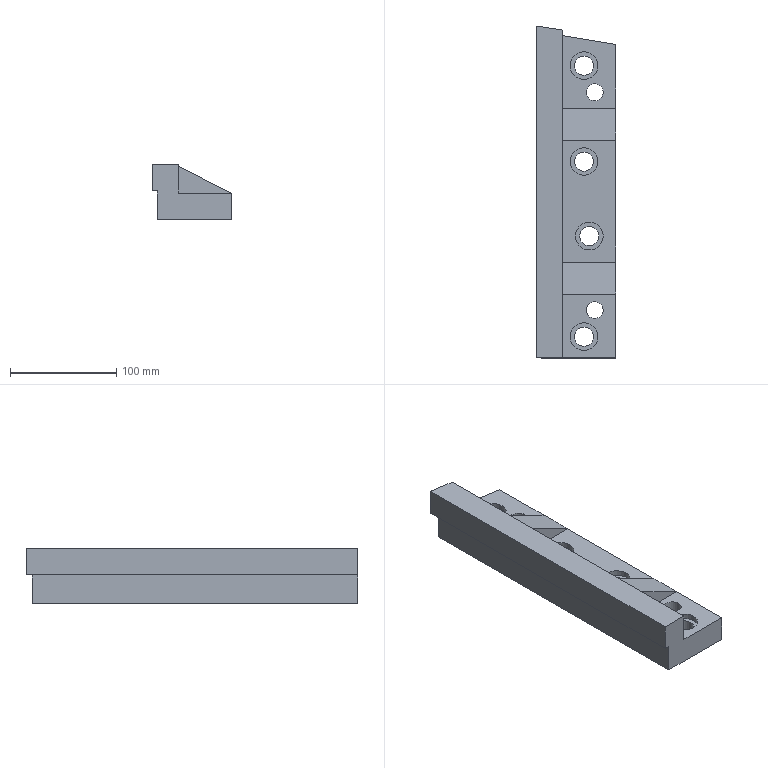Part | NX | features solid 2 | 1 solid | 33 faces | box 75 x 311.68 x 52 mm | volume 727777 mm3 | plane 21 | cylinder 10 | spline 2 | commonest cylinder face diameters 18 x4 26 x4 16 x2
STEP:
#1=CARTESIAN_POINT('',(-267.,-375.538,-30.));
#2=VERTEX_POINT('',#1);
#3=CARTESIAN_POINT('',(-280.,-375.538,-30.));
#4=DIRECTION('',(0.,0.,-1.));
#5=DIRECTION('',(1.,0.,0.));
#6=AXIS2_PLACEMENT_3D('',#3,#4,#5);
#7=CIRCLE('',#6,13.);
#8=EDGE_CURVE('',#2,#2,#7,.T.);
#9=ORIENTED_EDGE('',*,*,#8,.T.);
#10=EDGE_LOOP('',(#9));
#11=FACE_BOUND('',#10,.T.);
#12=CARTESIAN_POINT('',(-262.,-445.538,-30.));
#13=VERTEX_POINT('',#12);
#14=CARTESIAN_POINT('',(-275.,-445.538,-30.));
#15=DIRECTION('',(0.,0.,-1.));
#16=DIRECTION('',(1.,0.,0.));
#17=AXIS2_PLACEMENT_3D('',#14,#15,#16);
#18=CIRCLE('',#17,13.);
#19=EDGE_CURVE('',#13,#13,#18,.T.);
#20=ORIENTED_EDGE('',*,*,#19,.T.);
#21=EDGE_LOOP('',(#20));
#22=FACE_BOUND('',#21,.T.);
#23=CARTESIAN_POINT('',(-250.,-470.,-30.));
#24=VERTEX_POINT('',#23);
#25=CARTESIAN_POINT('',(-250.,-355.538,-30.));
#26=VERTEX_POINT('',#25);
#27=CARTESIAN_POINT('',(-250.,-560.,-30.));
#28=DIRECTION('',(0.,1.,0.));
#29=VECTOR('',#28,1000.);
#30=LINE('',#27,#29);
#31=EDGE_CURVE('',#24,#26,#30,.T.);
#32=ORIENTED_EDGE('',*,*,#31,.T.);
#33=CARTESIAN_POINT('',(-300.,-355.538,-30.));
#34=VERTEX_POINT('',#33);
#35=CARTESIAN_POINT('',(-300.,-355.538,-30.));
#36=DIRECTION('',(1.,0.,0.));
#37=VECTOR('',#36,1000.);
#38=LINE('',#35,#37);
#39=EDGE_CURVE('',#34,#26,#38,.T.);
#40=ORIENTED_EDGE('',*,*,#39,.F.);
#41=CARTESIAN_POINT('',(-300.,-470.,-30.));
#42=VERTEX_POINT('',#41);
#43=CARTESIAN_POINT('',(-300.,-560.,-30.));
#44=DIRECTION('',(0.,1.,0.));
#45=VECTOR('',#44,1000.);
#46=LINE('',#43,#45);
#47=EDGE_CURVE('',#42,#34,#46,.T.);
#48=ORIENTED_EDGE('',*,*,#47,.F.);
#49=CARTESIAN_POINT('',(-300.,-470.,-30.));
#50=DIRECTION('',(1.,0.,0.));
#51=VECTOR('',#50,1000.);
#52=LINE('',#49,#51);
#53=EDGE_CURVE('',#42,#24,#52,.T.);
#54=ORIENTED_EDGE('',*,*,#53,.T.);
#55=EDGE_LOOP('',(#32,#40,#48,#54));
#56=FACE_BOUND('',#55,.T.);
#57=CARTESIAN_POINT('',(-272.356,-257.29,-30.));
#58=DIRECTION('',(0.,0.,-1.));
#59=DIRECTION('',(-1.,0.,0.));
#60=AXIS2_PLACEMENT_3D('',#57,#58,#59);
#61=PLANE('',#60);
#62=ADVANCED_FACE('',(#11,#22,#56),#61,.F.);
#63=CARTESIAN_POINT('',(-267.,-285.538,-30.));
#64=VERTEX_POINT('',#63);
#65=CARTESIAN_POINT('',(-280.,-285.538,-30.));
#66=DIRECTION('',(0.,0.,-1.));
#67=DIRECTION('',(1.,0.,0.));
#68=AXIS2_PLACEMENT_3D('',#65,#66,#67);
#69=CIRCLE('',#68,13.);
#70=EDGE_CURVE('',#64,#64,#69,.T.);
#71=ORIENTED_EDGE('',*,*,#70,.T.);
#72=EDGE_LOOP('',(#71));
#73=FACE_BOUND('',#72,.T.);
#74=CARTESIAN_POINT('',(-262.,-310.538,-30.));
#75=VERTEX_POINT('',#74);
#76=CARTESIAN_POINT('',(-270.,-310.538,-30.));
#77=DIRECTION('',(0.,0.,-1.));
#78=DIRECTION('',(1.,0.,0.));
#79=AXIS2_PLACEMENT_3D('',#76,#77,#78);
#80=CIRCLE('',#79,8.);
#81=EDGE_CURVE('',#75,#75,#80,.T.);
#82=ORIENTED_EDGE('',*,*,#81,.T.);
#83=EDGE_LOOP('',(#82));
#84=FACE_BOUND('',#83,.T.);
#85=CARTESIAN_POINT('',(-300.,-325.538,-30.));
#86=VERTEX_POINT('',#85);
#87=CARTESIAN_POINT('',(-300.,-257.2,-30.));
#88=VERTEX_POINT('',#87);
#89=CARTESIAN_POINT('',(-300.,-560.,-30.));
#90=DIRECTION('',(0.,1.,0.));
#91=VECTOR('',#90,1000.);
#92=LINE('',#89,#91);
#93=EDGE_CURVE('',#86,#88,#92,.T.);
#94=ORIENTED_EDGE('',*,*,#93,.F.);
#95=CARTESIAN_POINT('',(-250.,-325.538,-30.));
#96=VERTEX_POINT('',#95);
#97=CARTESIAN_POINT('',(-300.,-325.538,-30.));
#98=DIRECTION('',(1.,0.,0.));
#99=VECTOR('',#98,1000.);
#100=LINE('',#97,#99);
#101=EDGE_CURVE('',#86,#96,#100,.T.);
#102=ORIENTED_EDGE('',*,*,#101,.T.);
#103=CARTESIAN_POINT('',(-250.,-265.538,-30.));
#104=VERTEX_POINT('',#103);
#105=CARTESIAN_POINT('',(-250.,-560.,-30.));
#106=DIRECTION('',(0.,1.,0.));
#107=VECTOR('',#106,1000.);
#108=LINE('',#105,#107);
#109=EDGE_CURVE('',#96,#104,#108,.T.);
#110=ORIENTED_EDGE('',*,*,#109,.T.);
#111=CARTESIAN_POINT('',(-250.,-265.538,-30.));
#112=CARTESIAN_POINT('',(-266.667,-262.759,-30.));
#113=CARTESIAN_POINT('',(-283.333,-259.979,-30.));
#114=CARTESIAN_POINT('',(-300.,-257.2,-30.));
#115=B_SPLINE_CURVE_WITH_KNOTS('',3,(#111,#112,#113,#114),.UNSPECIFIED.,.F.,.F.,(4,4),(0.3169,0.3676),.UNSPECIFIED.);
#116=EDGE_CURVE('',#104,#88,#115,.T.);
#117=ORIENTED_EDGE('',*,*,#116,.T.);
#118=EDGE_LOOP('',(#94,#102,#110,#117));
#119=FACE_BOUND('',#118,.T.);
#120=CARTESIAN_POINT('',(-272.356,-257.29,-30.));
#121=DIRECTION('',(0.,0.,-1.));
#122=DIRECTION('',(-1.,0.,0.));
#123=AXIS2_PLACEMENT_3D('',#120,#121,#122);
#124=PLANE('',#123);
#125=ADVANCED_FACE('',(#73,#84,#119),#124,.F.);
#126=CARTESIAN_POINT('',(-250.,-560.,-30.));
#127=VERTEX_POINT('',#126);
#128=CARTESIAN_POINT('',(-250.,-500.,-30.));
#129=VERTEX_POINT('',#128);
#130=CARTESIAN_POINT('',(-250.,-560.,-30.));
#131=DIRECTION('',(0.,1.,0.));
#132=VECTOR('',#131,1000.);
#133=LINE('',#130,#132);
#134=EDGE_CURVE('',#127,#129,#133,.T.);
#135=ORIENTED_EDGE('',*,*,#134,.T.);
#136=CARTESIAN_POINT('',(-300.,-500.,-30.));
#137=VERTEX_POINT('',#136);
#138=CARTESIAN_POINT('',(-300.,-500.,-30.));
#139=DIRECTION('',(1.,0.,0.));
#140=VECTOR('',#139,1000.);
#141=LINE('',#138,#140);
#142=EDGE_CURVE('',#137,#129,#141,.T.);
#143=ORIENTED_EDGE('',*,*,#142,.F.);
#144=CARTESIAN_POINT('',(-300.,-560.,-30.));
#145=VERTEX_POINT('',#144);
#146=CARTESIAN_POINT('',(-300.,-560.,-30.));
#147=DIRECTION('',(0.,1.,0.));
#148=VECTOR('',#147,1000.);
#149=LINE('',#146,#148);
#150=EDGE_CURVE('',#145,#137,#149,.T.);
#151=ORIENTED_EDGE('',*,*,#150,.F.);
#152=CARTESIAN_POINT('',(-245.,-560.,-30.));
#153=DIRECTION('',(-1.,0.,0.));
#154=VECTOR('',#153,1000.);
#155=LINE('',#152,#154);
#156=EDGE_CURVE('',#127,#145,#155,.T.);
#157=ORIENTED_EDGE('',*,*,#156,.F.);
#158=EDGE_LOOP('',(#135,#143,#151,#157));
#159=FACE_BOUND('',#158,.T.);
#160=CARTESIAN_POINT('',(-262.,-515.,-30.));
#161=VERTEX_POINT('',#160);
#162=CARTESIAN_POINT('',(-270.,-515.,-30.));
#163=DIRECTION('',(0.,0.,1.));
#164=DIRECTION('',(1.,0.,0.));
#165=AXIS2_PLACEMENT_3D('',#162,#163,#164);
#166=CIRCLE('',#165,8.);
#167=EDGE_CURVE('',#161,#161,#166,.T.);
#168=ORIENTED_EDGE('',*,*,#167,.F.);
#169=EDGE_LOOP('',(#168));
#170=FACE_BOUND('',#169,.T.);
#171=CARTESIAN_POINT('',(-267.,-540.,-30.));
#172=VERTEX_POINT('',#171);
#173=CARTESIAN_POINT('',(-280.,-540.,-30.));
#174=DIRECTION('',(0.,0.,1.));
#175=DIRECTION('',(1.,0.,0.));
#176=AXIS2_PLACEMENT_3D('',#173,#174,#175);
#177=CIRCLE('',#176,13.);
#178=EDGE_CURVE('',#172,#172,#177,.T.);
#179=ORIENTED_EDGE('',*,*,#178,.F.);
#180=EDGE_LOOP('',(#179));
#181=FACE_BOUND('',#180,.T.);
#182=CARTESIAN_POINT('',(-272.356,-257.29,-30.));
#183=DIRECTION('',(0.,0.,-1.));
#184=DIRECTION('',(-1.,0.,0.));
#185=AXIS2_PLACEMENT_3D('',#182,#183,#184);
#186=PLANE('',#185);
#187=ADVANCED_FACE('',(#159,#170,#181),#186,.F.);
#188=CARTESIAN_POINT('',(-289.,-540.,-55.));
#189=VERTEX_POINT('',#188);
#190=CARTESIAN_POINT('',(-280.,-540.,-55.));
#191=DIRECTION('',(0.,0.,-1.));
#192=DIRECTION('',(-1.,0.,0.));
#193=AXIS2_PLACEMENT_3D('',#190,#191,#192);
#194=CIRCLE('',#193,9.);
#195=EDGE_CURVE('',#189,#189,#194,.T.);
#196=ORIENTED_EDGE('',*,*,#195,.T.);
#197=EDGE_LOOP('',(#196));
#198=FACE_BOUND('',#197,.T.);
#199=CARTESIAN_POINT('',(-271.,-540.,-35.));
#200=VERTEX_POINT('',#199);
#201=CARTESIAN_POINT('',(-280.,-540.,-35.));
#202=DIRECTION('',(0.,0.,1.));
#203=DIRECTION('',(1.,0.,0.));
#204=AXIS2_PLACEMENT_3D('',#201,#202,#203);
#205=CIRCLE('',#204,9.);
#206=EDGE_CURVE('',#200,#200,#205,.F.);
#207=ORIENTED_EDGE('',*,*,#206,.F.);
#208=EDGE_LOOP('',(#207));
#209=FACE_BOUND('',#208,.T.);
#210=CARTESIAN_POINT('',(-280.,-540.,-60.));
#211=DIRECTION('',(0.,0.,1.));
#212=DIRECTION('',(1.,0.,0.));
#213=AXIS2_PLACEMENT_3D('',#210,#211,#212);
#214=CYLINDRICAL_SURFACE('',#213,9.);
#215=ADVANCED_FACE('',(#198,#209),#214,.F.);
#216=ORIENTED_EDGE('',*,*,#195,.F.);
#217=EDGE_LOOP('',(#216));
#218=FACE_BOUND('',#217,.T.);
#219=CARTESIAN_POINT('',(-278.,-515.,-55.));
#220=VERTEX_POINT('',#219);
#221=CARTESIAN_POINT('',(-270.,-515.,-55.));
#222=DIRECTION('',(0.,0.,-1.));
#223=DIRECTION('',(-1.,0.,0.));
#224=AXIS2_PLACEMENT_3D('',#221,#222,#223);
#225=CIRCLE('',#224,8.);
#226=EDGE_CURVE('',#220,#220,#225,.T.);
#227=ORIENTED_EDGE('',*,*,#226,.F.);
#228=EDGE_LOOP('',(#227));
#229=FACE_BOUND('',#228,.T.);
#230=CARTESIAN_POINT('',(-289.,-375.538,-55.));
#231=VERTEX_POINT('',#230);
#232=CARTESIAN_POINT('',(-280.,-375.538,-55.));
#233=DIRECTION('',(0.,0.,-1.));
#234=DIRECTION('',(-1.,0.,0.));
#235=AXIS2_PLACEMENT_3D('',#232,#233,#234);
#236=CIRCLE('',#235,9.);
#237=EDGE_CURVE('',#231,#231,#236,.F.);
#238=ORIENTED_EDGE('',*,*,#237,.T.);
#239=EDGE_LOOP('',(#238));
#240=FACE_BOUND('',#239,.T.);
#241=CARTESIAN_POINT('',(-289.,-285.538,-55.));
#242=VERTEX_POINT('',#241);
#243=CARTESIAN_POINT('',(-280.,-285.538,-55.));
#244=DIRECTION('',(0.,0.,-1.));
#245=DIRECTION('',(-1.,0.,0.));
#246=AXIS2_PLACEMENT_3D('',#243,#244,#245);
#247=CIRCLE('',#246,9.);
#248=EDGE_CURVE('',#242,#242,#247,.F.);
#249=ORIENTED_EDGE('',*,*,#248,.T.);
#250=EDGE_LOOP('',(#249));
#251=FACE_BOUND('',#250,.T.);
#252=CARTESIAN_POINT('',(-250.,-265.538,-55.));
#253=VERTEX_POINT('',#252);
#254=CARTESIAN_POINT('',(-320.,-254.082,-55.));
#255=VERTEX_POINT('',#254);
#256=CARTESIAN_POINT('',(-320.,-254.082,-55.));
#257=CARTESIAN_POINT('',(-318.477,-254.303,-55.));
#258=CARTESIAN_POINT('',(-315.46,-254.747,-55.));
#259=CARTESIAN_POINT('',(-311.763,-255.309,-55.));
#260=CARTESIAN_POINT('',(-308.848,-255.763,-55.));
#261=CARTESIAN_POINT('',(-306.685,-256.105,-55.));
#262=CARTESIAN_POINT('',(-304.9,-256.392,-55.));
#263=CARTESIAN_POINT('',(-303.484,-256.623,-55.));
#264=CARTESIAN_POINT('',(-302.6,-256.768,-55.));
#265=CARTESIAN_POINT('',(-301.992,-256.868,-55.));
#266=CARTESIAN_POINT('',(-301.633,-256.928,-55.));
#267=CARTESIAN_POINT('',(-301.436,-256.96,-55.));
#268=CARTESIAN_POINT('',(-301.216,-256.997,-55.));
#269=CARTESIAN_POINT('',(-301.227,-256.995,-55.));
#270=CARTESIAN_POINT('',(-301.202,-256.999,-55.));
#271=CARTESIAN_POINT('',(-301.151,-257.008,-55.));
#272=CARTESIAN_POINT('',(-300.987,-257.035,-55.));
#273=CARTESIAN_POINT('',(-300.565,-257.106,-55.));
#274=CARTESIAN_POINT('',(-299.722,-257.246,-55.));
#275=CARTESIAN_POINT('',(-298.214,-257.498,-55.));
#276=CARTESIAN_POINT('',(-296.206,-257.832,-55.));
#277=CARTESIAN_POINT('',(-293.699,-258.251,-55.));
#278=CARTESIAN_POINT('',(-291.193,-258.668,-55.));
#279=CARTESIAN_POINT('',(-288.94,-259.044,-55.));
#280=CARTESIAN_POINT('',(-287.122,-259.347,-55.));
#281=CARTESIAN_POINT('',(-285.514,-259.615,-55.));
#282=CARTESIAN_POINT('',(-284.14,-259.845,-55.));
#283=CARTESIAN_POINT('',(-283.314,-259.982,-55.));
#284=CARTESIAN_POINT('',(-282.503,-260.118,-55.));
#285=CARTESIAN_POINT('',(-282.171,-260.173,-55.));
#286=CARTESIAN_POINT('',(-281.513,-260.283,-55.));
#287=CARTESIAN_POINT('',(-280.252,-260.493,-55.));
#288=CARTESIAN_POINT('',(-278.422,-260.798,-55.));
#289=CARTESIAN_POINT('',(-276.238,-261.162,-55.));
#290=CARTESIAN_POINT('',(-274.051,-261.527,-55.));
#291=CARTESIAN_POINT('',(-271.136,-262.013,-55.));
#292=CARTESIAN_POINT('',(-267.492,-262.621,-55.));
#293=CARTESIAN_POINT('',(-263.119,-263.35,-55.));
#294=CARTESIAN_POINT('',(-257.288,-264.323,-55.));
#295=CARTESIAN_POINT('',(-252.915,-265.052,-55.));
#296=CARTESIAN_POINT('',(-250.,-265.538,-55.));
#297=B_SPLINE_CURVE_WITH_KNOTS('',3,(#256,#257,#258,#259,#260,#261,#262,#263,#264,#265,#266,#267,#268,#269,#270,#271,#272,#273,#274,#275,#276,#277,#278,#279,#280,#281,#282,#283,#284,#285,#286,#287,#288,#289,#290,#291,#292,#293,#294,#295,#296),.UNSPECIFIED.,.F.,.F.,(4,1,1,1,1,1,1,1,1,1,1,1,1,1,1,1,1,1,1,1,1,1,1,1,1,1,1,1,1,1,1,1,1,1,1,1,1,1,4),(0.,0.05833,0.1167,0.1458,0.175,0.2042,0.2187,0.2333,0.2406,0.2443,0.2479,0.2497,0.2516,0.2552,0.2625,0.2771,0.2917,0.3208,0.35,0.3792,0.4083,0.4375,0.4521,0.4667,0.4812,0.4885,0.4958,0.4995,0.5031,0.5104,0.525,0.5541,0.5833,0.6125,0.6416,0.7,0.7583,0.8166,0.9333),.UNSPECIFIED.);
#298=EDGE_CURVE('',#253,#255,#297,.F.);
#299=ORIENTED_EDGE('',*,*,#298,.F.);
#300=CARTESIAN_POINT('',(-250.,-560.,-55.));
#301=VERTEX_POINT('',#300);
#302=CARTESIAN_POINT('',(-250.,-560.,-55.));
#303=DIRECTION('',(0.,1.,0.));
#304=VECTOR('',#303,1000.);
#305=LINE('',#302,#304);
#306=EDGE_CURVE('',#301,#253,#305,.T.);
#307=ORIENTED_EDGE('',*,*,#306,.F.);
#308=CARTESIAN_POINT('',(-320.,-560.,-55.));
#309=VERTEX_POINT('',#308);
#310=CARTESIAN_POINT('',(-245.,-560.,-55.));
#311=DIRECTION('',(-1.,0.,0.));
#312=VECTOR('',#311,1000.);
#313=LINE('',#310,#312);
#314=EDGE_CURVE('',#301,#309,#313,.T.);
#315=ORIENTED_EDGE('',*,*,#314,.T.);
#316=CARTESIAN_POINT('',(-320.,-257.29,-55.));
#317=DIRECTION('',(0.,1.,0.));
#318=VECTOR('',#317,1000.);
#319=LINE('',#316,#318);
#320=EDGE_CURVE('',#309,#255,#319,.T.);
#321=ORIENTED_EDGE('',*,*,#320,.T.);
#322=EDGE_LOOP('',(#299,#307,#315,#321));
#323=FACE_BOUND('',#322,.T.);
#324=CARTESIAN_POINT('',(-278.,-310.538,-55.));
#325=VERTEX_POINT('',#324);
#326=CARTESIAN_POINT('',(-270.,-310.538,-55.));
#327=DIRECTION('',(0.,0.,-1.));
#328=DIRECTION('',(-1.,0.,0.));
#329=AXIS2_PLACEMENT_3D('',#326,#327,#328);
#330=CIRCLE('',#329,8.);
#331=EDGE_CURVE('',#325,#325,#330,.F.);
#332=ORIENTED_EDGE('',*,*,#331,.T.);
#333=EDGE_LOOP('',(#332));
#334=FACE_BOUND('',#333,.T.);
#335=CARTESIAN_POINT('',(-284.,-445.538,-55.));
#336=VERTEX_POINT('',#335);
#337=CARTESIAN_POINT('',(-275.,-445.538,-55.));
#338=DIRECTION('',(0.,0.,-1.));
#339=DIRECTION('',(-1.,0.,0.));
#340=AXIS2_PLACEMENT_3D('',#337,#338,#339);
#341=CIRCLE('',#340,9.);
#342=EDGE_CURVE('',#336,#336,#341,.F.);
#343=ORIENTED_EDGE('',*,*,#342,.T.);
#344=EDGE_LOOP('',(#343));
#345=FACE_BOUND('',#344,.T.);
#346=CARTESIAN_POINT('',(-272.356,-257.29,-55.));
#347=DIRECTION('',(0.,0.,-1.));
#348=DIRECTION('',(-1.,0.,0.));
#349=AXIS2_PLACEMENT_3D('',#346,#347,#348);
#350=PLANE('',#349);
#351=ADVANCED_FACE('',(#218,#229,#240,#251,#323,#334,#345),#350,.T.);
#352=CARTESIAN_POINT('',(-320.,-560.,-28.));
#353=VERTEX_POINT('',#352);
#354=CARTESIAN_POINT('',(-320.,-560.,-53.));
#355=DIRECTION('',(0.,0.,1.));
#356=VECTOR('',#355,1000.);
#357=LINE('',#354,#356);
#358=EDGE_CURVE('',#309,#353,#357,.T.);
#359=ORIENTED_EDGE('',*,*,#358,.F.);
#360=ORIENTED_EDGE('',*,*,#314,.F.);
#361=CARTESIAN_POINT('',(-250.,-560.,-53.));
#362=DIRECTION('',(0.,0.,1.));
#363=VECTOR('',#362,1000.);
#364=LINE('',#361,#363);
#365=EDGE_CURVE('',#301,#127,#364,.T.);
#366=ORIENTED_EDGE('',*,*,#365,.T.);
#367=ORIENTED_EDGE('',*,*,#156,.T.);
#368=CARTESIAN_POINT('',(-300.,-560.,-3.));
#369=VERTEX_POINT('',#368);
#370=CARTESIAN_POINT('',(-300.,-560.,-53.));
#371=DIRECTION('',(0.,0.,1.));
#372=VECTOR('',#371,1000.);
#373=LINE('',#370,#372);
#374=EDGE_CURVE('',#145,#369,#373,.T.);
#375=ORIENTED_EDGE('',*,*,#374,.T.);
#376=CARTESIAN_POINT('',(-325.,-560.,-3.));
#377=VERTEX_POINT('',#376);
#378=CARTESIAN_POINT('',(-300.,-560.,-3.));
#379=DIRECTION('',(-1.,0.,0.));
#380=VECTOR('',#379,1000.);
#381=LINE('',#378,#380);
#382=EDGE_CURVE('',#369,#377,#381,.T.);
#383=ORIENTED_EDGE('',*,*,#382,.T.);
#384=CARTESIAN_POINT('',(-325.,-560.,-28.));
#385=VERTEX_POINT('',#384);
#386=CARTESIAN_POINT('',(-325.,-560.,-53.));
#387=DIRECTION('',(0.,0.,1.));
#388=VECTOR('',#387,1000.);
#389=LINE('',#386,#388);
#390=EDGE_CURVE('',#385,#377,#389,.T.);
#391=ORIENTED_EDGE('',*,*,#390,.F.);
#392=CARTESIAN_POINT('',(-300.,-560.,-28.));
#393=DIRECTION('',(-1.,0.,0.));
#394=VECTOR('',#393,1000.);
#395=LINE('',#392,#394);
#396=EDGE_CURVE('',#353,#385,#395,.T.);
#397=ORIENTED_EDGE('',*,*,#396,.F.);
#398=EDGE_LOOP('',(#359,#360,#366,#367,#375,#383,#391,#397));
#399=FACE_BOUND('',#398,.T.);
#400=CARTESIAN_POINT('',(-245.,-560.,-53.));
#401=DIRECTION('',(0.,1.,0.));
#402=DIRECTION('',(0.,0.,1.));
#403=AXIS2_PLACEMENT_3D('',#400,#401,#402);
#404=PLANE('',#403);
#405=ADVANCED_FACE('',(#399),#404,.F.);
#406=CARTESIAN_POINT('',(-325.,-248.32,-28.));
#407=VERTEX_POINT('',#406);
#408=CARTESIAN_POINT('',(-325.,-248.32,-3.));
#409=VERTEX_POINT('',#408);
#410=CARTESIAN_POINT('',(-325.,-248.32,-53.));
#411=DIRECTION('',(0.,0.,1.));
#412=VECTOR('',#411,1000.);
#413=LINE('',#410,#412);
#414=EDGE_CURVE('',#407,#409,#413,.T.);
#415=ORIENTED_EDGE('',*,*,#414,.F.);
#416=CARTESIAN_POINT('',(-325.,-560.,-28.));
#417=DIRECTION('',(0.,1.,0.));
#418=VECTOR('',#417,1000.);
#419=LINE('',#416,#418);
#420=EDGE_CURVE('',#385,#407,#419,.T.);
#421=ORIENTED_EDGE('',*,*,#420,.F.);
#422=ORIENTED_EDGE('',*,*,#390,.T.);
#423=CARTESIAN_POINT('',(-325.,-560.,-3.));
#424=DIRECTION('',(0.,1.,0.));
#425=VECTOR('',#424,1000.);
#426=LINE('',#423,#425);
#427=EDGE_CURVE('',#377,#409,#426,.T.);
#428=ORIENTED_EDGE('',*,*,#427,.T.);
#429=EDGE_LOOP('',(#415,#421,#422,#428));
#430=FACE_BOUND('',#429,.T.);
#431=CARTESIAN_POINT('',(-325.,-560.,-53.));
#432=DIRECTION('',(1.,0.,0.));
#433=DIRECTION('',(0.,0.,-1.));
#434=AXIS2_PLACEMENT_3D('',#431,#432,#433);
#435=PLANE('',#434);
#436=ADVANCED_FACE('',(#430),#435,.F.);
#437=CARTESIAN_POINT('',(-250.,-265.538,-42.5));
#438=DIRECTION('',(0.,0.,-1.));
#439=VECTOR('',#438,1000.);
#440=LINE('',#437,#439);
#441=EDGE_CURVE('',#104,#253,#440,.T.);
#442=ORIENTED_EDGE('',*,*,#441,.F.);
#443=ORIENTED_EDGE('',*,*,#109,.F.);
#444=CARTESIAN_POINT('',(-250.,-355.538,-30.));
#445=DIRECTION('',(0.,1.,0.));
#446=VECTOR('',#445,1000.);
#447=LINE('',#444,#446);
#448=EDGE_CURVE('',#26,#96,#447,.T.);
#449=ORIENTED_EDGE('',*,*,#448,.F.);
#450=ORIENTED_EDGE('',*,*,#31,.F.);
#451=CARTESIAN_POINT('',(-250.,-470.,-30.));
#452=DIRECTION('',(0.,-1.,0.));
#453=VECTOR('',#452,1000.);
#454=LINE('',#451,#453);
#455=EDGE_CURVE('',#24,#129,#454,.T.);
#456=ORIENTED_EDGE('',*,*,#455,.T.);
#457=ORIENTED_EDGE('',*,*,#134,.F.);
#458=ORIENTED_EDGE('',*,*,#365,.F.);
#459=ORIENTED_EDGE('',*,*,#306,.T.);
#460=EDGE_LOOP('',(#442,#443,#449,#450,#456,#457,#458,#459));
#461=FACE_BOUND('',#460,.T.);
#462=CARTESIAN_POINT('',(-250.,-560.,-53.));
#463=DIRECTION('',(1.,0.,0.));
#464=DIRECTION('',(0.,0.,-1.));
#465=AXIS2_PLACEMENT_3D('',#462,#463,#464);
#466=PLANE('',#465);
#467=ADVANCED_FACE('',(#461),#466,.T.);
#468=CARTESIAN_POINT('',(-300.,-355.538,-5.));
#469=VERTEX_POINT('',#468);
#470=CARTESIAN_POINT('',(-300.,-355.538,-30.));
#471=DIRECTION('',(0.,0.,1.));
#472=VECTOR('',#471,1000.);
#473=LINE('',#470,#472);
#474=EDGE_CURVE('',#34,#469,#473,.T.);
#475=ORIENTED_EDGE('',*,*,#474,.T.);
#476=CARTESIAN_POINT('',(-300.,-325.538,-5.));
#477=VERTEX_POINT('',#476);
#478=CARTESIAN_POINT('',(-300.,-355.538,-5.));
#479=DIRECTION('',(0.,-1.,0.));
#480=VECTOR('',#479,1000.);
#481=LINE('',#478,#480);
#482=EDGE_CURVE('',#469,#477,#481,.F.);
#483=ORIENTED_EDGE('',*,*,#482,.T.);
#484=CARTESIAN_POINT('',(-300.,-325.538,-30.));
#485=DIRECTION('',(0.,0.,1.));
#486=VECTOR('',#485,1000.);
#487=LINE('',#484,#486);
#488=EDGE_CURVE('',#86,#477,#487,.T.);
#489=ORIENTED_EDGE('',*,*,#488,.F.);
#490=ORIENTED_EDGE('',*,*,#93,.T.);
#491=CARTESIAN_POINT('',(-300.,-257.2,-28.));
#492=VERTEX_POINT('',#491);
#493=CARTESIAN_POINT('',(-300.,-257.2,-28.));
#494=DIRECTION('',(0.,0.,-1.));
#495=VECTOR('',#494,1000.);
#496=LINE('',#493,#495);
#497=EDGE_CURVE('',#492,#88,#496,.T.);
#498=ORIENTED_EDGE('',*,*,#497,.F.);
#499=CARTESIAN_POINT('',(-300.,-252.131,-28.));
#500=VERTEX_POINT('',#499);
#501=CARTESIAN_POINT('',(-300.,-560.,-28.));
#502=DIRECTION('',(0.,-1.,0.));
#503=VECTOR('',#502,1000.);
#504=LINE('',#501,#503);
#505=EDGE_CURVE('',#500,#492,#504,.T.);
#506=ORIENTED_EDGE('',*,*,#505,.F.);
#507=CARTESIAN_POINT('',(-300.,-252.131,-3.));
#508=VERTEX_POINT('',#507);
#509=CARTESIAN_POINT('',(-300.,-252.131,-53.));
#510=DIRECTION('',(0.,0.,1.));
#511=VECTOR('',#510,1000.);
#512=LINE('',#509,#511);
#513=EDGE_CURVE('',#500,#508,#512,.T.);
#514=ORIENTED_EDGE('',*,*,#513,.T.);
#515=CARTESIAN_POINT('',(-300.,-560.,-3.));
#516=DIRECTION('',(0.,1.,0.));
#517=VECTOR('',#516,1000.);
#518=LINE('',#515,#517);
#519=EDGE_CURVE('',#369,#508,#518,.T.);
#520=ORIENTED_EDGE('',*,*,#519,.F.);
#521=ORIENTED_EDGE('',*,*,#374,.F.);
#522=ORIENTED_EDGE('',*,*,#150,.T.);
#523=CARTESIAN_POINT('',(-300.,-500.,-5.));
#524=VERTEX_POINT('',#523);
#525=CARTESIAN_POINT('',(-300.,-500.,-30.));
#526=DIRECTION('',(0.,0.,1.));
#527=VECTOR('',#526,1000.);
#528=LINE('',#525,#527);
#529=EDGE_CURVE('',#137,#524,#528,.T.);
#530=ORIENTED_EDGE('',*,*,#529,.T.);
#531=CARTESIAN_POINT('',(-300.,-470.,-5.));
#532=VERTEX_POINT('',#531);
#533=CARTESIAN_POINT('',(-300.,-470.,-5.));
#534=DIRECTION('',(0.,1.,0.));
#535=VECTOR('',#534,1000.);
#536=LINE('',#533,#535);
#537=EDGE_CURVE('',#532,#524,#536,.F.);
#538=ORIENTED_EDGE('',*,*,#537,.F.);
#539=CARTESIAN_POINT('',(-300.,-470.,-30.));
#540=DIRECTION('',(0.,0.,1.));
#541=VECTOR('',#540,1000.);
#542=LINE('',#539,#541);
#543=EDGE_CURVE('',#42,#532,#542,.T.);
#544=ORIENTED_EDGE('',*,*,#543,.F.);
#545=ORIENTED_EDGE('',*,*,#47,.T.);
#546=EDGE_LOOP('',(#475,#483,#489,#490,#498,#506,#514,#520,#521,#522,#530,#538,#544,#545));
#547=FACE_BOUND('',#546,.T.);
#548=CARTESIAN_POINT('',(-300.,-560.,-53.));
#549=DIRECTION('',(1.,0.,0.));
#550=DIRECTION('',(0.,0.,-1.));
#551=AXIS2_PLACEMENT_3D('',#548,#549,#550);
#552=PLANE('',#551);
#553=ADVANCED_FACE('',(#547),#552,.T.);
#554=ORIENTED_EDGE('',*,*,#513,.F.);
#555=CARTESIAN_POINT('',(-300.,-252.131,-28.));
#556=CARTESIAN_POINT('',(-308.316,-250.744,-28.));
#557=CARTESIAN_POINT('',(-316.652,-249.486,-28.));
#558=CARTESIAN_POINT('',(-325.,-248.32,-28.));
#559=B_SPLINE_CURVE_WITH_KNOTS('',3,(#555,#556,#557,#558),.UNSPECIFIED.,.F.,.F.,(4,4),(0.,1.),.PIECEWISE_BEZIER_KNOTS.);
#560=EDGE_CURVE('',#407,#500,#559,.F.);
#561=ORIENTED_EDGE('',*,*,#560,.F.);
#562=ORIENTED_EDGE('',*,*,#414,.T.);
#563=CARTESIAN_POINT('',(-300.,-252.131,-3.));
#564=CARTESIAN_POINT('',(-308.316,-250.744,-3.));
#565=CARTESIAN_POINT('',(-316.652,-249.486,-3.));
#566=CARTESIAN_POINT('',(-325.,-248.32,-3.));
#567=B_SPLINE_CURVE_WITH_KNOTS('',3,(#563,#564,#565,#566),.UNSPECIFIED.,.F.,.F.,(4,4),(0.,1.),.PIECEWISE_BEZIER_KNOTS.);
#568=EDGE_CURVE('',#508,#409,#567,.T.);
#569=ORIENTED_EDGE('',*,*,#568,.F.);
#570=EDGE_LOOP('',(#554,#561,#562,#569));
#571=FACE_BOUND('',#570,.T.);
#572=CARTESIAN_POINT('',(-300.,-252.131,-28.));
#573=CARTESIAN_POINT('',(-300.,-252.131,-3.));
#574=CARTESIAN_POINT('',(-308.316,-250.744,-28.));
#575=CARTESIAN_POINT('',(-308.316,-250.744,-3.));
#576=CARTESIAN_POINT('',(-316.652,-249.486,-28.));
#577=CARTESIAN_POINT('',(-316.652,-249.486,-3.));
#578=CARTESIAN_POINT('',(-325.,-248.32,-28.));
#579=CARTESIAN_POINT('',(-325.,-248.32,-3.));
#580=B_SPLINE_SURFACE_WITH_KNOTS('',3,1,((#572,#573),(#574,#575),(#576,#577),(#578,#579)),.SURF_OF_LINEAR_EXTRUSION.,.F.,.F.,.F.,(4,4),(2,2),(0.,1.),(0.,1.),.PIECEWISE_BEZIER_KNOTS.);
#581=ADVANCED_FACE('',(#571),#580,.T.);
#582=ORIENTED_EDGE('',*,*,#519,.T.);
#583=ORIENTED_EDGE('',*,*,#568,.T.);
#584=ORIENTED_EDGE('',*,*,#427,.F.);
#585=ORIENTED_EDGE('',*,*,#382,.F.);
#586=EDGE_LOOP('',(#582,#583,#584,#585));
#587=FACE_BOUND('',#586,.T.);
#588=CARTESIAN_POINT('',(-312.488,-250.142,-3.));
#589=DIRECTION('',(0.,0.,-1.));
#590=DIRECTION('',(-1.,0.,0.));
#591=AXIS2_PLACEMENT_3D('',#588,#589,#590);
#592=PLANE('',#591);
#593=ADVANCED_FACE('',(#587),#592,.F.);
#594=ORIENTED_EDGE('',*,*,#420,.T.);
#595=ORIENTED_EDGE('',*,*,#560,.T.);
#596=ORIENTED_EDGE('',*,*,#505,.T.);
#597=CARTESIAN_POINT('',(-320.,-254.082,-28.));
#598=VERTEX_POINT('',#597);
#599=CARTESIAN_POINT('',(-300.,-257.2,-28.));
#600=CARTESIAN_POINT('',(-306.691,-256.084,-28.));
#601=CARTESIAN_POINT('',(-313.32,-255.051,-28.));
#602=CARTESIAN_POINT('',(-320.,-254.082,-28.));
#603=B_SPLINE_CURVE_WITH_KNOTS('',3,(#599,#600,#601,#602),.UNSPECIFIED.,.F.,.F.,(4,4),(-0.03297,0.7716),.UNSPECIFIED.);
#604=EDGE_CURVE('',#492,#598,#603,.T.);
#605=ORIENTED_EDGE('',*,*,#604,.T.);
#606=CARTESIAN_POINT('',(-320.,-560.,-28.));
#607=DIRECTION('',(0.,1.,0.));
#608=VECTOR('',#607,1000.);
#609=LINE('',#606,#608);
#610=EDGE_CURVE('',#353,#598,#609,.T.);
#611=ORIENTED_EDGE('',*,*,#610,.F.);
#612=ORIENTED_EDGE('',*,*,#396,.T.);
#613=EDGE_LOOP('',(#594,#595,#596,#605,#611,#612));
#614=FACE_BOUND('',#613,.T.);
#615=CARTESIAN_POINT('',(-300.,-560.,-28.));
#616=DIRECTION('',(0.,0.,-1.));
#617=DIRECTION('',(-1.,0.,0.));
#618=AXIS2_PLACEMENT_3D('',#615,#616,#617);
#619=PLANE('',#618);
#620=ADVANCED_FACE('',(#614),#619,.T.);
#621=CARTESIAN_POINT('',(-320.,-254.082,-40.5));
#622=DIRECTION('',(0.,0.,-1.));
#623=VECTOR('',#622,1000.);
#624=LINE('',#621,#623);
#625=EDGE_CURVE('',#255,#598,#624,.F.);
#626=ORIENTED_EDGE('',*,*,#625,.F.);
#627=ORIENTED_EDGE('',*,*,#320,.F.);
#628=ORIENTED_EDGE('',*,*,#358,.T.);
#629=ORIENTED_EDGE('',*,*,#610,.T.);
#630=EDGE_LOOP('',(#626,#627,#628,#629));
#631=FACE_BOUND('',#630,.T.);
#632=CARTESIAN_POINT('',(-320.,-560.,-28.));
#633=DIRECTION('',(-1.,0.,0.));
#634=DIRECTION('',(0.,0.,1.));
#635=AXIS2_PLACEMENT_3D('',#632,#633,#634);
#636=PLANE('',#635);
#637=ADVANCED_FACE('',(#631),#636,.T.);
#638=ORIENTED_EDGE('',*,*,#441,.T.);
#639=ORIENTED_EDGE('',*,*,#298,.T.);
#640=ORIENTED_EDGE('',*,*,#625,.T.);
#641=ORIENTED_EDGE('',*,*,#604,.F.);
#642=ORIENTED_EDGE('',*,*,#497,.T.);
#643=ORIENTED_EDGE('',*,*,#116,.F.);
#644=EDGE_LOOP('',(#638,#639,#640,#641,#642,#643));
#645=FACE_BOUND('',#644,.T.);
#646=CARTESIAN_POINT('',(-250.,-265.538,-28.));
#647=CARTESIAN_POINT('',(-250.,-265.538,-55.));
#648=CARTESIAN_POINT('',(-261.679,-263.591,-28.));
#649=CARTESIAN_POINT('',(-261.679,-263.591,-55.));
#650=CARTESIAN_POINT('',(-279.191,-260.693,-28.));
#651=CARTESIAN_POINT('',(-279.191,-260.693,-55.));
#652=CARTESIAN_POINT('',(-302.566,-256.734,-28.));
#653=CARTESIAN_POINT('',(-302.566,-256.734,-55.));
#654=CARTESIAN_POINT('',(-314.17,-254.927,-28.));
#655=CARTESIAN_POINT('',(-314.17,-254.927,-55.));
#656=CARTESIAN_POINT('',(-320.,-254.082,-28.));
#657=CARTESIAN_POINT('',(-320.,-254.082,-55.));
#658=B_SPLINE_SURFACE_WITH_KNOTS('',3,1,((#646,#647),(#648,#649),(#650,#651),(#652,#653),(#654,#655),(#656,#657)),.SURF_OF_LINEAR_EXTRUSION.,.F.,.F.,.F.,(4,1,1,4),(2,2),(-2.037,-0.6327,0.06946,0.7716),(0.,1.),.UNSPECIFIED.);
#659=ADVANCED_FACE('',(#645),#658,.F.);
#660=CARTESIAN_POINT('',(-289.,-285.538,-35.));
#661=VERTEX_POINT('',#660);
#662=CARTESIAN_POINT('',(-280.,-285.538,-35.));
#663=DIRECTION('',(0.,0.,-1.));
#664=DIRECTION('',(-1.,0.,0.));
#665=AXIS2_PLACEMENT_3D('',#662,#663,#664);
#666=CIRCLE('',#665,9.);
#667=EDGE_CURVE('',#661,#661,#666,.T.);
#668=ORIENTED_EDGE('',*,*,#667,.F.);
#669=EDGE_LOOP('',(#668));
#670=FACE_BOUND('',#669,.T.);
#671=ORIENTED_EDGE('',*,*,#248,.F.);
#672=EDGE_LOOP('',(#671));
#673=FACE_BOUND('',#672,.T.);
#674=CARTESIAN_POINT('',(-280.,-285.538,-60.));
#675=DIRECTION('',(0.,0.,1.));
#676=DIRECTION('',(1.,0.,0.));
#677=AXIS2_PLACEMENT_3D('',#674,#675,#676);
#678=CYLINDRICAL_SURFACE('',#677,9.);
#679=ADVANCED_FACE('',(#670,#673),#678,.F.);
#680=ORIENTED_EDGE('',*,*,#331,.F.);
#681=EDGE_LOOP('',(#680));
#682=FACE_BOUND('',#681,.T.);
#683=ORIENTED_EDGE('',*,*,#81,.F.);
#684=EDGE_LOOP('',(#683));
#685=FACE_BOUND('',#684,.T.);
#686=CARTESIAN_POINT('',(-270.,-310.538,-60.));
#687=DIRECTION('',(0.,0.,1.));
#688=DIRECTION('',(1.,0.,0.));
#689=AXIS2_PLACEMENT_3D('',#686,#687,#688);
#690=CYLINDRICAL_SURFACE('',#689,8.);
#691=ADVANCED_FACE('',(#682,#685),#690,.F.);
#692=CARTESIAN_POINT('',(-289.,-375.538,-35.));
#693=VERTEX_POINT('',#692);
#694=CARTESIAN_POINT('',(-280.,-375.538,-35.));
#695=DIRECTION('',(0.,0.,-1.));
#696=DIRECTION('',(-1.,0.,0.));
#697=AXIS2_PLACEMENT_3D('',#694,#695,#696);
#698=CIRCLE('',#697,9.);
#699=EDGE_CURVE('',#693,#693,#698,.T.);
#700=ORIENTED_EDGE('',*,*,#699,.F.);
#701=EDGE_LOOP('',(#700));
#702=FACE_BOUND('',#701,.T.);
#703=ORIENTED_EDGE('',*,*,#237,.F.);
#704=EDGE_LOOP('',(#703));
#705=FACE_BOUND('',#704,.T.);
#706=CARTESIAN_POINT('',(-280.,-375.538,-60.));
#707=DIRECTION('',(0.,0.,1.));
#708=DIRECTION('',(1.,0.,0.));
#709=AXIS2_PLACEMENT_3D('',#706,#707,#708);
#710=CYLINDRICAL_SURFACE('',#709,9.);
#711=ADVANCED_FACE('',(#702,#705),#710,.F.);
#712=CARTESIAN_POINT('',(-284.,-445.538,-35.));
#713=VERTEX_POINT('',#712);
#714=CARTESIAN_POINT('',(-275.,-445.538,-35.));
#715=DIRECTION('',(0.,0.,-1.));
#716=DIRECTION('',(-1.,0.,0.));
#717=AXIS2_PLACEMENT_3D('',#714,#715,#716);
#718=CIRCLE('',#717,9.);
#719=EDGE_CURVE('',#713,#713,#718,.T.);
#720=ORIENTED_EDGE('',*,*,#719,.F.);
#721=EDGE_LOOP('',(#720));
#722=FACE_BOUND('',#721,.T.);
#723=ORIENTED_EDGE('',*,*,#342,.F.);
#724=EDGE_LOOP('',(#723));
#725=FACE_BOUND('',#724,.T.);
#726=CARTESIAN_POINT('',(-275.,-445.538,-60.));
#727=DIRECTION('',(0.,0.,1.));
#728=DIRECTION('',(1.,0.,0.));
#729=AXIS2_PLACEMENT_3D('',#726,#727,#728);
#730=CYLINDRICAL_SURFACE('',#729,9.);
#731=ADVANCED_FACE('',(#722,#725),#730,.F.);
#732=ORIENTED_EDGE('',*,*,#226,.T.);
#733=EDGE_LOOP('',(#732));
#734=FACE_BOUND('',#733,.T.);
#735=ORIENTED_EDGE('',*,*,#167,.T.);
#736=EDGE_LOOP('',(#735));
#737=FACE_BOUND('',#736,.T.);
#738=CARTESIAN_POINT('',(-270.,-515.,-60.));
#739=DIRECTION('',(0.,0.,1.));
#740=DIRECTION('',(1.,0.,0.));
#741=AXIS2_PLACEMENT_3D('',#738,#739,#740);
#742=CYLINDRICAL_SURFACE('',#741,8.);
#743=ADVANCED_FACE('',(#734,#737),#742,.F.);
#744=CARTESIAN_POINT('',(-267.,-540.,-35.));
#745=VERTEX_POINT('',#744);
#746=CARTESIAN_POINT('',(-280.,-540.,-35.));
#747=DIRECTION('',(0.,0.,1.));
#748=DIRECTION('',(1.,0.,0.));
#749=AXIS2_PLACEMENT_3D('',#746,#747,#748);
#750=CIRCLE('',#749,13.);
#751=EDGE_CURVE('',#745,#745,#750,.T.);
#752=ORIENTED_EDGE('',*,*,#751,.T.);
#753=EDGE_LOOP('',(#752));
#754=FACE_BOUND('',#753,.T.);
#755=ORIENTED_EDGE('',*,*,#206,.T.);
#756=EDGE_LOOP('',(#755));
#757=FACE_BOUND('',#756,.T.);
#758=CARTESIAN_POINT('',(-280.,-540.,-35.));
#759=DIRECTION('',(0.,0.,1.));
#760=DIRECTION('',(1.,0.,0.));
#761=AXIS2_PLACEMENT_3D('',#758,#759,#760);
#762=PLANE('',#761);
#763=ADVANCED_FACE('',(#754,#757),#762,.T.);
#764=ORIENTED_EDGE('',*,*,#751,.F.);
#765=EDGE_LOOP('',(#764));
#766=FACE_BOUND('',#765,.T.);
#767=ORIENTED_EDGE('',*,*,#178,.T.);
#768=EDGE_LOOP('',(#767));
#769=FACE_BOUND('',#768,.T.);
#770=CARTESIAN_POINT('',(-280.,-540.,-35.));
#771=DIRECTION('',(0.,0.,1.));
#772=DIRECTION('',(1.,0.,0.));
#773=AXIS2_PLACEMENT_3D('',#770,#771,#772);
#774=CYLINDRICAL_SURFACE('',#773,13.);
#775=ADVANCED_FACE('',(#766,#769),#774,.F.);
#776=CARTESIAN_POINT('',(-262.,-445.538,-35.));
#777=VERTEX_POINT('',#776);
#778=CARTESIAN_POINT('',(-275.,-445.538,-35.));
#779=DIRECTION('',(0.,0.,-1.));
#780=DIRECTION('',(1.,0.,0.));
#781=AXIS2_PLACEMENT_3D('',#778,#779,#780);
#782=CIRCLE('',#781,13.);
#783=EDGE_CURVE('',#777,#777,#782,.T.);
#784=ORIENTED_EDGE('',*,*,#783,.T.);
#785=EDGE_LOOP('',(#784));
#786=FACE_BOUND('',#785,.T.);
#787=ORIENTED_EDGE('',*,*,#19,.F.);
#788=EDGE_LOOP('',(#787));
#789=FACE_BOUND('',#788,.T.);
#790=CARTESIAN_POINT('',(-275.,-445.538,-35.));
#791=DIRECTION('',(0.,0.,1.));
#792=DIRECTION('',(1.,0.,0.));
#793=AXIS2_PLACEMENT_3D('',#790,#791,#792);
#794=CYLINDRICAL_SURFACE('',#793,13.);
#795=ADVANCED_FACE('',(#786,#789),#794,.F.);
#796=ORIENTED_EDGE('',*,*,#719,.T.);
#797=EDGE_LOOP('',(#796));
#798=FACE_BOUND('',#797,.T.);
#799=ORIENTED_EDGE('',*,*,#783,.F.);
#800=EDGE_LOOP('',(#799));
#801=FACE_BOUND('',#800,.T.);
#802=CARTESIAN_POINT('',(-275.,-445.538,-35.));
#803=DIRECTION('',(0.,0.,-1.));
#804=DIRECTION('',(-1.,0.,0.));
#805=AXIS2_PLACEMENT_3D('',#802,#803,#804);
#806=PLANE('',#805);
#807=ADVANCED_FACE('',(#798,#801),#806,.F.);
#808=CARTESIAN_POINT('',(-267.,-375.538,-35.));
#809=VERTEX_POINT('',#808);
#810=CARTESIAN_POINT('',(-280.,-375.538,-35.));
#811=DIRECTION('',(0.,0.,-1.));
#812=DIRECTION('',(1.,0.,0.));
#813=AXIS2_PLACEMENT_3D('',#810,#811,#812);
#814=CIRCLE('',#813,13.);
#815=EDGE_CURVE('',#809,#809,#814,.T.);
#816=ORIENTED_EDGE('',*,*,#815,.T.);
#817=EDGE_LOOP('',(#816));
#818=FACE_BOUND('',#817,.T.);
#819=ORIENTED_EDGE('',*,*,#8,.F.);
#820=EDGE_LOOP('',(#819));
#821=FACE_BOUND('',#820,.T.);
#822=CARTESIAN_POINT('',(-280.,-375.538,-35.));
#823=DIRECTION('',(0.,0.,1.));
#824=DIRECTION('',(1.,0.,0.));
#825=AXIS2_PLACEMENT_3D('',#822,#823,#824);
#826=CYLINDRICAL_SURFACE('',#825,13.);
#827=ADVANCED_FACE('',(#818,#821),#826,.F.);
#828=ORIENTED_EDGE('',*,*,#699,.T.);
#829=EDGE_LOOP('',(#828));
#830=FACE_BOUND('',#829,.T.);
#831=ORIENTED_EDGE('',*,*,#815,.F.);
#832=EDGE_LOOP('',(#831));
#833=FACE_BOUND('',#832,.T.);
#834=CARTESIAN_POINT('',(-280.,-375.538,-35.));
#835=DIRECTION('',(0.,0.,-1.));
#836=DIRECTION('',(-1.,0.,0.));
#837=AXIS2_PLACEMENT_3D('',#834,#835,#836);
#838=PLANE('',#837);
#839=ADVANCED_FACE('',(#830,#833),#838,.F.);
#840=CARTESIAN_POINT('',(-267.,-285.538,-35.));
#841=VERTEX_POINT('',#840);
#842=CARTESIAN_POINT('',(-280.,-285.538,-35.));
#843=DIRECTION('',(0.,0.,-1.));
#844=DIRECTION('',(1.,0.,0.));
#845=AXIS2_PLACEMENT_3D('',#842,#843,#844);
#846=CIRCLE('',#845,13.);
#847=EDGE_CURVE('',#841,#841,#846,.T.);
#848=ORIENTED_EDGE('',*,*,#847,.T.);
#849=EDGE_LOOP('',(#848));
#850=FACE_BOUND('',#849,.T.);
#851=ORIENTED_EDGE('',*,*,#70,.F.);
#852=EDGE_LOOP('',(#851));
#853=FACE_BOUND('',#852,.T.);
#854=CARTESIAN_POINT('',(-280.,-285.538,-35.));
#855=DIRECTION('',(0.,0.,1.));
#856=DIRECTION('',(1.,0.,0.));
#857=AXIS2_PLACEMENT_3D('',#854,#855,#856);
#858=CYLINDRICAL_SURFACE('',#857,13.);
#859=ADVANCED_FACE('',(#850,#853),#858,.F.);
#860=ORIENTED_EDGE('',*,*,#667,.T.);
#861=EDGE_LOOP('',(#860));
#862=FACE_BOUND('',#861,.T.);
#863=ORIENTED_EDGE('',*,*,#847,.F.);
#864=EDGE_LOOP('',(#863));
#865=FACE_BOUND('',#864,.T.);
#866=CARTESIAN_POINT('',(-280.,-285.538,-35.));
#867=DIRECTION('',(0.,0.,-1.));
#868=DIRECTION('',(-1.,0.,0.));
#869=AXIS2_PLACEMENT_3D('',#866,#867,#868);
#870=PLANE('',#869);
#871=ADVANCED_FACE('',(#862,#865),#870,.F.);
#872=ORIENTED_EDGE('',*,*,#543,.T.);
#873=CARTESIAN_POINT('',(-290.,-470.,-10.));
#874=DIRECTION('',(0.8944,0.,-0.4472));
#875=VECTOR('',#874,1000.);
#876=LINE('',#873,#875);
#877=EDGE_CURVE('',#532,#24,#876,.T.);
#878=ORIENTED_EDGE('',*,*,#877,.T.);
#879=ORIENTED_EDGE('',*,*,#53,.F.);
#880=EDGE_LOOP('',(#872,#878,#879));
#881=FACE_BOUND('',#880,.T.);
#882=CARTESIAN_POINT('',(-300.,-470.,-30.));
#883=DIRECTION('',(0.,1.,0.));
#884=DIRECTION('',(1.,0.,0.));
#885=AXIS2_PLACEMENT_3D('',#882,#883,#884);
#886=PLANE('',#885);
#887=ADVANCED_FACE('',(#881),#886,.T.);
#888=ORIENTED_EDGE('',*,*,#142,.T.);
#889=CARTESIAN_POINT('',(-290.,-500.,-10.));
#890=DIRECTION('',(0.8944,0.,-0.4472));
#891=VECTOR('',#890,1000.);
#892=LINE('',#889,#891);
#893=EDGE_CURVE('',#129,#524,#892,.F.);
#894=ORIENTED_EDGE('',*,*,#893,.T.);
#895=ORIENTED_EDGE('',*,*,#529,.F.);
#896=EDGE_LOOP('',(#888,#894,#895));
#897=FACE_BOUND('',#896,.T.);
#898=CARTESIAN_POINT('',(-300.,-500.,-30.));
#899=DIRECTION('',(0.,1.,0.));
#900=DIRECTION('',(1.,0.,0.));
#901=AXIS2_PLACEMENT_3D('',#898,#899,#900);
#902=PLANE('',#901);
#903=ADVANCED_FACE('',(#897),#902,.F.);
#904=ORIENTED_EDGE('',*,*,#877,.F.);
#905=ORIENTED_EDGE('',*,*,#537,.T.);
#906=ORIENTED_EDGE('',*,*,#893,.F.);
#907=ORIENTED_EDGE('',*,*,#455,.F.);
#908=EDGE_LOOP('',(#904,#905,#906,#907));
#909=FACE_BOUND('',#908,.T.);
#910=CARTESIAN_POINT('',(-250.,-470.,-30.));
#911=DIRECTION('',(0.4472,0.,0.8944));
#912=DIRECTION('',(0.8944,0.,-0.4472));
#913=AXIS2_PLACEMENT_3D('',#910,#911,#912);
#914=PLANE('',#913);
#915=ADVANCED_FACE('',(#909),#914,.T.);
#916=ORIENTED_EDGE('',*,*,#39,.T.);
#917=CARTESIAN_POINT('',(-290.,-355.538,-10.));
#918=DIRECTION('',(-0.8944,0.,0.4472));
#919=VECTOR('',#918,1000.);
#920=LINE('',#917,#919);
#921=EDGE_CURVE('',#26,#469,#920,.T.);
#922=ORIENTED_EDGE('',*,*,#921,.T.);
#923=ORIENTED_EDGE('',*,*,#474,.F.);
#924=EDGE_LOOP('',(#916,#922,#923));
#925=FACE_BOUND('',#924,.T.);
#926=CARTESIAN_POINT('',(-300.,-355.538,-30.));
#927=DIRECTION('',(0.,-1.,0.));
#928=DIRECTION('',(1.,0.,0.));
#929=AXIS2_PLACEMENT_3D('',#926,#927,#928);
#930=PLANE('',#929);
#931=ADVANCED_FACE('',(#925),#930,.T.);
#932=ORIENTED_EDGE('',*,*,#488,.T.);
#933=CARTESIAN_POINT('',(-290.,-325.538,-10.));
#934=DIRECTION('',(-0.8944,0.,0.4472));
#935=VECTOR('',#934,1000.);
#936=LINE('',#933,#935);
#937=EDGE_CURVE('',#477,#96,#936,.F.);
#938=ORIENTED_EDGE('',*,*,#937,.T.);
#939=ORIENTED_EDGE('',*,*,#101,.F.);
#940=EDGE_LOOP('',(#932,#938,#939));
#941=FACE_BOUND('',#940,.T.);
#942=CARTESIAN_POINT('',(-300.,-325.538,-30.));
#943=DIRECTION('',(0.,-1.,0.));
#944=DIRECTION('',(1.,0.,0.));
#945=AXIS2_PLACEMENT_3D('',#942,#943,#944);
#946=PLANE('',#945);
#947=ADVANCED_FACE('',(#941),#946,.F.);
#948=ORIENTED_EDGE('',*,*,#921,.F.);
#949=ORIENTED_EDGE('',*,*,#448,.T.);
#950=ORIENTED_EDGE('',*,*,#937,.F.);
#951=ORIENTED_EDGE('',*,*,#482,.F.);
#952=EDGE_LOOP('',(#948,#949,#950,#951));
#953=FACE_BOUND('',#952,.T.);
#954=CARTESIAN_POINT('',(-300.,-355.538,-5.));
#955=DIRECTION('',(0.4472,0.,0.8944));
#956=DIRECTION('',(0.8944,0.,-0.4472));
#957=AXIS2_PLACEMENT_3D('',#954,#955,#956);
#958=PLANE('',#957);
#959=ADVANCED_FACE('',(#953),#958,.T.);
#960=CLOSED_SHELL('',(#62,#125,#187,#215,#351,#405,#436,#467,#553,#581,#593,#620,#637,#659,#679,#691,#711,#731,#743,#763,#775,#795,#807,#827,#839,#859,#871,#887,#903,#915,#931,#947,#959));
#961=MANIFOLD_SOLID_BREP('',#960);
#962=(LENGTH_UNIT()NAMED_UNIT(*)SI_UNIT(.MILLI.,.METRE.));
#963=UNCERTAINTY_MEASURE_WITH_UNIT(LENGTH_MEASURE(0.0508),#962,'','');
#964=(NAMED_UNIT(*)PLANE_ANGLE_UNIT()SI_UNIT($,.RADIAN.));
#965=(NAMED_UNIT(*)SI_UNIT($,.STERADIAN.)SOLID_ANGLE_UNIT());
#966=(GEOMETRIC_REPRESENTATION_CONTEXT(3)GLOBAL_UNCERTAINTY_ASSIGNED_CONTEXT((#963))GLOBAL_UNIT_ASSIGNED_CONTEXT((#962,#964,#965))REPRESENTATION_CONTEXT('',''));
#967=ADVANCED_BREP_SHAPE_REPRESENTATION('',(#961),#966);